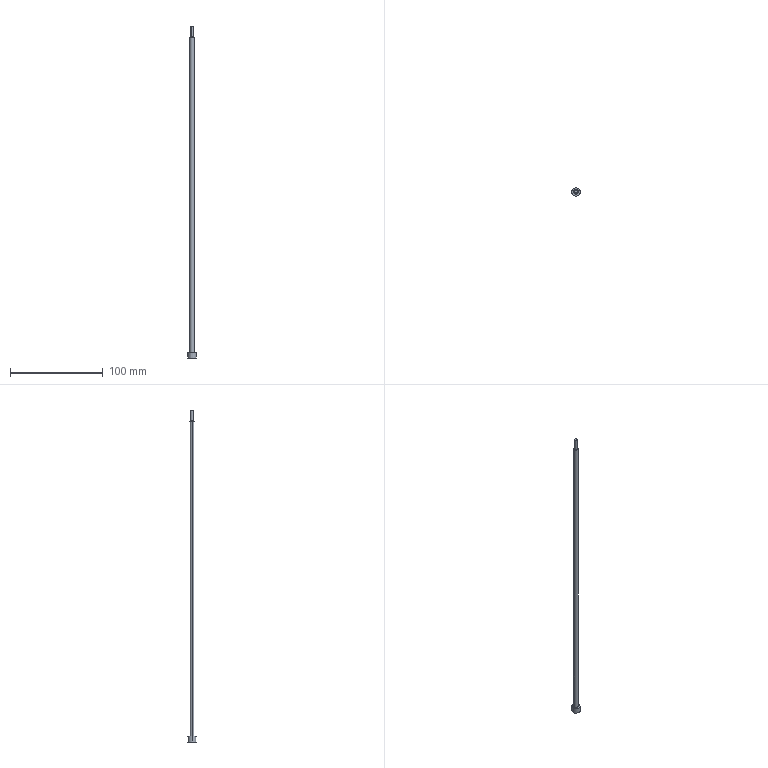Part | Creo | 1 solid | 12 faces | box 9 x 9 x 357.548 mm | volume 5878 mm3 | cylinder 6 | plane 4 | cone 2 | commonest cylinder face diameters 3.214 x2 4.5 x2 9 x2
STEP:
#1=CARTESIAN_POINT('',(79.096,-142.631,-319.5));
#2=VERTEX_POINT('',#1);
#3=CARTESIAN_POINT('',(83.596,-142.631,-319.5));
#4=VERTEX_POINT('',#3);
#5=CARTESIAN_POINT('',(81.346,-142.631,-319.5));
#6=DIRECTION('',(0.,0.,-1.));
#7=DIRECTION('',(-1.,0.,0.));
#8=AXIS2_PLACEMENT_3D('',#5,#6,#7);
#9=CIRCLE('',#8,2.25);
#10=EDGE_CURVE('',#2,#4,#9,.T.);
#11=ORIENTED_EDGE('',*,*,#10,.T.);
#12=CARTESIAN_POINT('',(83.596,-142.631,19.789));
#13=VERTEX_POINT('',#12);
#14=CARTESIAN_POINT('',(83.596,-142.631,-319.5));
#15=DIRECTION('',(0.,0.,1.));
#16=VECTOR('',#15,339.289);
#17=LINE('',#14,#16);
#18=EDGE_CURVE('',#4,#13,#17,.T.);
#19=ORIENTED_EDGE('',*,*,#18,.T.);
#20=CARTESIAN_POINT('',(79.096,-142.631,19.789));
#21=VERTEX_POINT('',#20);
#22=CARTESIAN_POINT('',(81.346,-142.631,19.789));
#23=DIRECTION('',(0.,0.,1.));
#24=DIRECTION('',(1.,0.,0.));
#25=AXIS2_PLACEMENT_3D('',#22,#23,#24);
#26=CIRCLE('',#25,2.25);
#27=EDGE_CURVE('',#13,#21,#26,.T.);
#28=ORIENTED_EDGE('',*,*,#27,.T.);
#29=CARTESIAN_POINT('',(79.096,-142.631,-319.5));
#30=DIRECTION('',(0.,0.,1.));
#31=VECTOR('',#30,339.289);
#32=LINE('',#29,#31);
#33=EDGE_CURVE('',#2,#21,#32,.T.);
#34=ORIENTED_EDGE('',*,*,#33,.F.);
#35=EDGE_LOOP('',(#11,#19,#28,#34));
#36=FACE_OUTER_BOUND('',#35,.F.);
#37=CARTESIAN_POINT('',(81.346,-142.631,-310.5));
#38=DIRECTION('',(0.,0.,1.));
#39=DIRECTION('',(1.,0.,0.));
#40=AXIS2_PLACEMENT_3D('',#37,#38,#39);
#41=CYLINDRICAL_SURFACE('',#40,2.25);
#42=ADVANCED_FACE('',(#36),#41,.T.);
#43=CARTESIAN_POINT('',(76.846,-142.631,-319.5));
#44=VERTEX_POINT('',#43);
#45=CARTESIAN_POINT('',(85.846,-142.631,-319.5));
#46=VERTEX_POINT('',#45);
#47=CARTESIAN_POINT('',(81.346,-142.631,-319.5));
#48=DIRECTION('',(0.,0.,1.));
#49=DIRECTION('',(-1.,0.,0.));
#50=AXIS2_PLACEMENT_3D('',#47,#48,#49);
#51=CIRCLE('',#50,4.5);
#52=EDGE_CURVE('',#44,#46,#51,.T.);
#53=ORIENTED_EDGE('',*,*,#52,.F.);
#54=CARTESIAN_POINT('',(81.346,-142.631,-319.5));
#55=DIRECTION('',(0.,0.,1.));
#56=DIRECTION('',(1.,0.,0.));
#57=AXIS2_PLACEMENT_3D('',#54,#55,#56);
#58=CIRCLE('',#57,4.5);
#59=EDGE_CURVE('',#46,#44,#58,.T.);
#60=ORIENTED_EDGE('',*,*,#59,.F.);
#61=EDGE_LOOP('',(#53,#60));
#62=FACE_OUTER_BOUND('',#61,.F.);
#63=CARTESIAN_POINT('',(81.346,-142.631,-319.5));
#64=DIRECTION('',(0.,0.,-1.));
#65=DIRECTION('',(1.,0.,0.));
#66=AXIS2_PLACEMENT_3D('',#63,#64,#65);
#67=CIRCLE('',#66,2.25);
#68=EDGE_CURVE('',#4,#2,#67,.T.);
#69=ORIENTED_EDGE('',*,*,#68,.F.);
#70=ORIENTED_EDGE('',*,*,#10,.F.);
#71=EDGE_LOOP('',(#69,#70));
#72=FACE_BOUND('',#71,.F.);
#73=CARTESIAN_POINT('',(81.346,-142.631,-319.5));
#74=DIRECTION('',(0.,0.,1.));
#75=DIRECTION('',(1.,0.,0.));
#76=AXIS2_PLACEMENT_3D('',#73,#74,#75);
#77=PLANE('',#76);
#78=ADVANCED_FACE('',(#62,#72),#77,.T.);
#79=ORIENTED_EDGE('',*,*,#68,.T.);
#80=ORIENTED_EDGE('',*,*,#33,.T.);
#81=CARTESIAN_POINT('',(81.346,-142.631,19.789));
#82=DIRECTION('',(0.,0.,1.));
#83=DIRECTION('',(-1.,0.,0.));
#84=AXIS2_PLACEMENT_3D('',#81,#82,#83);
#85=CIRCLE('',#84,2.25);
#86=EDGE_CURVE('',#21,#13,#85,.T.);
#87=ORIENTED_EDGE('',*,*,#86,.T.);
#88=ORIENTED_EDGE('',*,*,#18,.F.);
#89=EDGE_LOOP('',(#79,#80,#87,#88));
#90=FACE_OUTER_BOUND('',#89,.F.);
#91=CARTESIAN_POINT('',(81.346,-142.631,-310.5));
#92=DIRECTION('',(0.,0.,1.));
#93=DIRECTION('',(1.,0.,0.));
#94=AXIS2_PLACEMENT_3D('',#91,#92,#93);
#95=CYLINDRICAL_SURFACE('',#94,2.25);
#96=ADVANCED_FACE('',(#90),#95,.T.);
#97=ORIENTED_EDGE('',*,*,#86,.F.);
#98=ORIENTED_EDGE('',*,*,#27,.F.);
#99=EDGE_LOOP('',(#97,#98));
#100=FACE_OUTER_BOUND('',#99,.F.);
#101=CARTESIAN_POINT('',(81.346,-140.522,19.789));
#102=VERTEX_POINT('',#101);
#103=CARTESIAN_POINT('',(83.455,-142.631,19.789));
#104=VERTEX_POINT('',#103);
#105=CARTESIAN_POINT('',(81.346,-142.631,19.789));
#106=DIRECTION('',(0.,0.,-1.));
#107=DIRECTION('',(0.,1.,0.));
#108=AXIS2_PLACEMENT_3D('',#105,#106,#107);
#109=CIRCLE('',#108,2.109);
#110=EDGE_CURVE('',#102,#104,#109,.T.);
#111=ORIENTED_EDGE('',*,*,#110,.F.);
#112=CARTESIAN_POINT('',(79.237,-142.631,19.789));
#113=VERTEX_POINT('',#112);
#114=CARTESIAN_POINT('',(81.346,-142.631,19.789));
#115=DIRECTION('',(0.,0.,-1.));
#116=DIRECTION('',(-1.,0.,0.));
#117=AXIS2_PLACEMENT_3D('',#114,#115,#116);
#118=CIRCLE('',#117,2.109);
#119=EDGE_CURVE('',#113,#102,#118,.T.);
#120=ORIENTED_EDGE('',*,*,#119,.F.);
#121=CARTESIAN_POINT('',(81.346,-142.631,19.789));
#122=DIRECTION('',(0.,0.,-1.));
#123=DIRECTION('',(1.,0.,0.));
#124=AXIS2_PLACEMENT_3D('',#121,#122,#123);
#125=CIRCLE('',#124,2.109);
#126=EDGE_CURVE('',#104,#113,#125,.T.);
#127=ORIENTED_EDGE('',*,*,#126,.F.);
#128=EDGE_LOOP('',(#111,#120,#127));
#129=FACE_BOUND('',#128,.F.);
#130=CARTESIAN_POINT('',(-0.003698,-18.777,19.789));
#131=DIRECTION('',(0.,0.,-1.));
#132=DIRECTION('',(0.,-1.,0.));
#133=AXIS2_PLACEMENT_3D('',#130,#131,#132);
#134=PLANE('',#133);
#135=ADVANCED_FACE('',(#100,#129),#134,.F.);
#136=CARTESIAN_POINT('',(81.346,-141.024,20.291));
#137=VERTEX_POINT('',#136);
#138=CARTESIAN_POINT('',(82.953,-142.631,20.291));
#139=VERTEX_POINT('',#138);
#140=CARTESIAN_POINT('',(81.346,-142.631,20.291));
#141=DIRECTION('',(0.,0.,-1.));
#142=DIRECTION('',(0.,1.,0.));
#143=AXIS2_PLACEMENT_3D('',#140,#141,#142);
#144=CIRCLE('',#143,1.607);
#145=EDGE_CURVE('',#137,#139,#144,.T.);
#146=ORIENTED_EDGE('',*,*,#145,.F.);
#147=CARTESIAN_POINT('',(79.739,-142.631,20.291));
#148=VERTEX_POINT('',#147);
#149=CARTESIAN_POINT('',(81.346,-142.631,20.291));
#150=DIRECTION('',(0.,0.,-1.));
#151=DIRECTION('',(-1.,0.,0.));
#152=AXIS2_PLACEMENT_3D('',#149,#150,#151);
#153=CIRCLE('',#152,1.607);
#154=EDGE_CURVE('',#148,#137,#153,.T.);
#155=ORIENTED_EDGE('',*,*,#154,.F.);
#156=CARTESIAN_POINT('',(79.739,-142.631,20.291));
#157=DIRECTION('',(-0.7071,0.,-0.7072));
#158=VECTOR('',#157,0.7099);
#159=LINE('',#156,#158);
#160=EDGE_CURVE('',#148,#113,#159,.T.);
#161=ORIENTED_EDGE('',*,*,#160,.T.);
#162=ORIENTED_EDGE('',*,*,#119,.T.);
#163=ORIENTED_EDGE('',*,*,#110,.T.);
#164=CARTESIAN_POINT('',(82.953,-142.631,20.291));
#165=DIRECTION('',(0.7071,0.,-0.7072));
#166=VECTOR('',#165,0.7099);
#167=LINE('',#164,#166);
#168=EDGE_CURVE('',#139,#104,#167,.T.);
#169=ORIENTED_EDGE('',*,*,#168,.F.);
#170=EDGE_LOOP('',(#146,#155,#161,#162,#163,#169));
#171=FACE_OUTER_BOUND('',#170,.F.);
#172=CARTESIAN_POINT('',(81.346,-142.631,20.04));
#173=DIRECTION('',(0.,0.,-1.));
#174=DIRECTION('',(1.,0.,0.));
#175=AXIS2_PLACEMENT_3D('',#172,#173,#174);
#176=CONICAL_SURFACE('',#175,1.858,44.996);
#177=ADVANCED_FACE('',(#171),#176,.T.);
#178=CARTESIAN_POINT('',(81.346,-144.239,31.987));
#179=VERTEX_POINT('',#178);
#180=CARTESIAN_POINT('',(82.953,-142.631,31.926));
#181=VERTEX_POINT('',#180);
#182=CARTESIAN_POINT('',(81.346,-144.239,31.987));
#183=CARTESIAN_POINT('',(81.565,-144.239,31.979));
#184=CARTESIAN_POINT('',(81.969,-144.156,31.963));
#185=CARTESIAN_POINT('',(82.509,-143.803,31.943));
#186=CARTESIAN_POINT('',(82.867,-143.263,31.929));
#187=CARTESIAN_POINT('',(82.953,-142.854,31.926));
#188=B_SPLINE_CURVE_WITH_KNOTS('',3,(#182,#183,#184,#185,#186,#187,#180),.UNSPECIFIED.,.F.,.F.,(4,1,1,1,4),(0.,0.25,0.5,0.75,1.),.UNSPECIFIED.);
#189=EDGE_CURVE('',#179,#181,#188,.T.);
#190=ORIENTED_EDGE('',*,*,#189,.T.);
#191=CARTESIAN_POINT('',(81.346,-141.024,31.987));
#192=VERTEX_POINT('',#191);
#193=CARTESIAN_POINT('',(82.953,-142.631,31.926));
#194=CARTESIAN_POINT('',(82.953,-142.409,31.926));
#195=CARTESIAN_POINT('',(82.867,-142.,31.929));
#196=CARTESIAN_POINT('',(82.509,-141.46,31.943));
#197=CARTESIAN_POINT('',(81.969,-141.107,31.963));
#198=CARTESIAN_POINT('',(81.565,-141.024,31.979));
#199=CARTESIAN_POINT('',(81.346,-141.024,31.987));
#200=B_SPLINE_CURVE_WITH_KNOTS('',3,(#193,#194,#195,#196,#197,#198,#199),.UNSPECIFIED.,.F.,.F.,(4,1,1,1,4),(0.,0.25,0.5,0.75,1.),.UNSPECIFIED.);
#201=EDGE_CURVE('',#181,#192,#200,.T.);
#202=ORIENTED_EDGE('',*,*,#201,.T.);
#203=CARTESIAN_POINT('',(81.346,-141.024,31.987));
#204=DIRECTION('',(-0.000004501,0.000001249,-1.));
#205=VECTOR('',#204,11.696);
#206=LINE('',#203,#205);
#207=EDGE_CURVE('',#192,#137,#206,.T.);
#208=ORIENTED_EDGE('',*,*,#207,.T.);
#209=ORIENTED_EDGE('',*,*,#145,.T.);
#210=CARTESIAN_POINT('',(81.346,-144.239,20.291));
#211=VERTEX_POINT('',#210);
#212=CARTESIAN_POINT('',(81.346,-142.631,20.291));
#213=DIRECTION('',(0.,0.,-1.));
#214=DIRECTION('',(1.,0.,0.));
#215=AXIS2_PLACEMENT_3D('',#212,#213,#214);
#216=CIRCLE('',#215,1.607);
#217=EDGE_CURVE('',#139,#211,#216,.T.);
#218=ORIENTED_EDGE('',*,*,#217,.T.);
#219=CARTESIAN_POINT('',(81.346,-144.239,31.987));
#220=DIRECTION('',(0.,-0.000001249,-1.));
#221=VECTOR('',#220,11.696);
#222=LINE('',#219,#221);
#223=EDGE_CURVE('',#179,#211,#222,.T.);
#224=ORIENTED_EDGE('',*,*,#223,.F.);
#225=EDGE_LOOP('',(#190,#202,#208,#209,#218,#224));
#226=FACE_OUTER_BOUND('',#225,.F.);
#227=CARTESIAN_POINT('',(81.346,-142.631,19.789));
#228=DIRECTION('',(0.,0.,-1.));
#229=DIRECTION('',(0.,-1.,0.));
#230=AXIS2_PLACEMENT_3D('',#227,#228,#229);
#231=CYLINDRICAL_SURFACE('',#230,1.607);
#232=ADVANCED_FACE('',(#226),#231,.T.);
#233=CARTESIAN_POINT('',(79.739,-142.631,32.048));
#234=VERTEX_POINT('',#233);
#235=CARTESIAN_POINT('',(81.346,-141.024,31.987));
#236=CARTESIAN_POINT('',(81.127,-141.024,31.995));
#237=CARTESIAN_POINT('',(80.724,-141.107,32.011));
#238=CARTESIAN_POINT('',(80.183,-141.46,32.031));
#239=CARTESIAN_POINT('',(79.825,-142.,32.045));
#240=CARTESIAN_POINT('',(79.739,-142.409,32.048));
#241=CARTESIAN_POINT('',(79.739,-142.631,32.048));
#242=B_SPLINE_CURVE_WITH_KNOTS('',3,(#235,#236,#237,#238,#239,#240,#241),.UNSPECIFIED.,.F.,.F.,(4,1,1,1,4),(0.,0.25,0.5,0.75,1.),.UNSPECIFIED.);
#243=EDGE_CURVE('',#192,#234,#242,.T.);
#244=ORIENTED_EDGE('',*,*,#243,.F.);
#245=ORIENTED_EDGE('',*,*,#201,.F.);
#246=ORIENTED_EDGE('',*,*,#189,.F.);
#247=CARTESIAN_POINT('',(79.739,-142.809,32.048));
#248=CARTESIAN_POINT('',(79.795,-143.142,32.046));
#249=CARTESIAN_POINT('',(80.029,-143.597,32.037));
#250=CARTESIAN_POINT('',(80.389,-143.955,32.024));
#251=CARTESIAN_POINT('',(80.845,-144.185,32.006));
#252=CARTESIAN_POINT('',(81.173,-144.239,31.994));
#253=CARTESIAN_POINT('',(81.346,-144.239,31.987));
#254=B_SPLINE_CURVE_WITH_KNOTS('',3,(#233,#247,#248,#249,#250,#251,#252,#253),.UNSPECIFIED.,.F.,.F.,(4,1,1,1,1,4),(0.,0.2,0.4,0.6,0.8,1.),.UNSPECIFIED.);
#255=EDGE_CURVE('',#234,#179,#254,.T.);
#256=ORIENTED_EDGE('',*,*,#255,.F.);
#257=EDGE_LOOP('',(#244,#245,#246,#256));
#258=FACE_OUTER_BOUND('',#257,.F.);
#259=CARTESIAN_POINT('',(-122.791,-167.242,39.779));
#260=DIRECTION('',(-0.03814,0.,-0.9993));
#261=DIRECTION('',(-0.9993,0.,0.03814));
#262=AXIS2_PLACEMENT_3D('',#259,#260,#261);
#263=PLANE('',#262);
#264=ADVANCED_FACE('',(#258),#263,.F.);
#265=ORIENTED_EDGE('',*,*,#255,.T.);
#266=ORIENTED_EDGE('',*,*,#223,.T.);
#267=CARTESIAN_POINT('',(81.346,-142.631,20.291));
#268=DIRECTION('',(0.,0.,-1.));
#269=DIRECTION('',(0.,-1.,0.));
#270=AXIS2_PLACEMENT_3D('',#267,#268,#269);
#271=CIRCLE('',#270,1.607);
#272=EDGE_CURVE('',#211,#148,#271,.T.);
#273=ORIENTED_EDGE('',*,*,#272,.T.);
#274=ORIENTED_EDGE('',*,*,#154,.T.);
#275=ORIENTED_EDGE('',*,*,#207,.F.);
#276=ORIENTED_EDGE('',*,*,#243,.T.);
#277=EDGE_LOOP('',(#265,#266,#273,#274,#275,#276));
#278=FACE_OUTER_BOUND('',#277,.F.);
#279=CARTESIAN_POINT('',(81.346,-142.631,19.789));
#280=DIRECTION('',(0.,0.,-1.));
#281=DIRECTION('',(0.,-1.,0.));
#282=AXIS2_PLACEMENT_3D('',#279,#280,#281);
#283=CYLINDRICAL_SURFACE('',#282,1.607);
#284=ADVANCED_FACE('',(#278),#283,.T.);
#285=ORIENTED_EDGE('',*,*,#217,.F.);
#286=ORIENTED_EDGE('',*,*,#168,.T.);
#287=ORIENTED_EDGE('',*,*,#126,.T.);
#288=ORIENTED_EDGE('',*,*,#160,.F.);
#289=ORIENTED_EDGE('',*,*,#272,.F.);
#290=EDGE_LOOP('',(#285,#286,#287,#288,#289));
#291=FACE_OUTER_BOUND('',#290,.F.);
#292=CARTESIAN_POINT('',(81.346,-142.631,20.04));
#293=DIRECTION('',(0.,0.,-1.));
#294=DIRECTION('',(1.,0.,0.));
#295=AXIS2_PLACEMENT_3D('',#292,#293,#294);
#296=CONICAL_SURFACE('',#295,1.858,44.996);
#297=ADVANCED_FACE('',(#291),#296,.T.);
#298=ORIENTED_EDGE('',*,*,#52,.T.);
#299=CARTESIAN_POINT('',(85.846,-142.631,-325.5));
#300=VERTEX_POINT('',#299);
#301=CARTESIAN_POINT('',(85.846,-142.631,-325.5));
#302=DIRECTION('',(0.,0.,1.));
#303=VECTOR('',#302,6.);
#304=LINE('',#301,#303);
#305=EDGE_CURVE('',#300,#46,#304,.T.);
#306=ORIENTED_EDGE('',*,*,#305,.F.);
#307=CARTESIAN_POINT('',(76.846,-142.631,-325.5));
#308=VERTEX_POINT('',#307);
#309=CARTESIAN_POINT('',(81.346,-142.631,-325.5));
#310=DIRECTION('',(0.,0.,-1.));
#311=DIRECTION('',(1.,0.,0.));
#312=AXIS2_PLACEMENT_3D('',#309,#310,#311);
#313=CIRCLE('',#312,4.5);
#314=EDGE_CURVE('',#300,#308,#313,.T.);
#315=ORIENTED_EDGE('',*,*,#314,.T.);
#316=CARTESIAN_POINT('',(76.846,-142.631,-325.5));
#317=DIRECTION('',(0.,0.,1.));
#318=VECTOR('',#317,6.);
#319=LINE('',#316,#318);
#320=EDGE_CURVE('',#308,#44,#319,.T.);
#321=ORIENTED_EDGE('',*,*,#320,.T.);
#322=EDGE_LOOP('',(#298,#306,#315,#321));
#323=FACE_OUTER_BOUND('',#322,.F.);
#324=CARTESIAN_POINT('',(81.346,-142.631,-325.5));
#325=DIRECTION('',(0.,0.,1.));
#326=DIRECTION('',(1.,0.,0.));
#327=AXIS2_PLACEMENT_3D('',#324,#325,#326);
#328=CYLINDRICAL_SURFACE('',#327,4.5);
#329=ADVANCED_FACE('',(#323),#328,.T.);
#330=ORIENTED_EDGE('',*,*,#59,.T.);
#331=ORIENTED_EDGE('',*,*,#320,.F.);
#332=CARTESIAN_POINT('',(81.346,-142.631,-325.5));
#333=DIRECTION('',(0.,0.,-1.));
#334=DIRECTION('',(-1.,0.,0.));
#335=AXIS2_PLACEMENT_3D('',#332,#333,#334);
#336=CIRCLE('',#335,4.5);
#337=EDGE_CURVE('',#308,#300,#336,.T.);
#338=ORIENTED_EDGE('',*,*,#337,.T.);
#339=ORIENTED_EDGE('',*,*,#305,.T.);
#340=EDGE_LOOP('',(#330,#331,#338,#339));
#341=FACE_OUTER_BOUND('',#340,.F.);
#342=CARTESIAN_POINT('',(81.346,-142.631,-325.5));
#343=DIRECTION('',(0.,0.,1.));
#344=DIRECTION('',(1.,0.,0.));
#345=AXIS2_PLACEMENT_3D('',#342,#343,#344);
#346=CYLINDRICAL_SURFACE('',#345,4.5);
#347=ADVANCED_FACE('',(#341),#346,.T.);
#348=ORIENTED_EDGE('',*,*,#314,.F.);
#349=ORIENTED_EDGE('',*,*,#337,.F.);
#350=EDGE_LOOP('',(#348,#349));
#351=FACE_OUTER_BOUND('',#350,.F.);
#352=CARTESIAN_POINT('',(81.346,-142.631,-325.5));
#353=DIRECTION('',(0.,0.,-1.));
#354=DIRECTION('',(-1.,0.,0.));
#355=AXIS2_PLACEMENT_3D('',#352,#353,#354);
#356=PLANE('',#355);
#357=ADVANCED_FACE('',(#351),#356,.T.);
#358=CLOSED_SHELL('',(#42,#78,#96,#135,#177,#232,#264,#284,#297,#329,#347,#357));
#359=MANIFOLD_SOLID_BREP('',#358);
#360=(LENGTH_UNIT()NAMED_UNIT(*)SI_UNIT(.MILLI.,.METRE.));
#361=UNCERTAINTY_MEASURE_WITH_UNIT(LENGTH_MEASURE(0.03578),#360,'','');
#362=(NAMED_UNIT(*)PLANE_ANGLE_UNIT()SI_UNIT($,.RADIAN.));
#363=PLANE_ANGLE_MEASURE_WITH_UNIT(PLANE_ANGLE_MEASURE(0.01745),#362);
#364=(CONVERSION_BASED_UNIT('DEGREE',#363)NAMED_UNIT(*)PLANE_ANGLE_UNIT());
#365=(NAMED_UNIT(*)SI_UNIT($,.STERADIAN.)SOLID_ANGLE_UNIT());
#366=(GEOMETRIC_REPRESENTATION_CONTEXT(3)GLOBAL_UNCERTAINTY_ASSIGNED_CONTEXT((#361))GLOBAL_UNIT_ASSIGNED_CONTEXT((#360,#364,#365))REPRESENTATION_CONTEXT('',''));
#367=ADVANCED_BREP_SHAPE_REPRESENTATION('',(#359),#366);